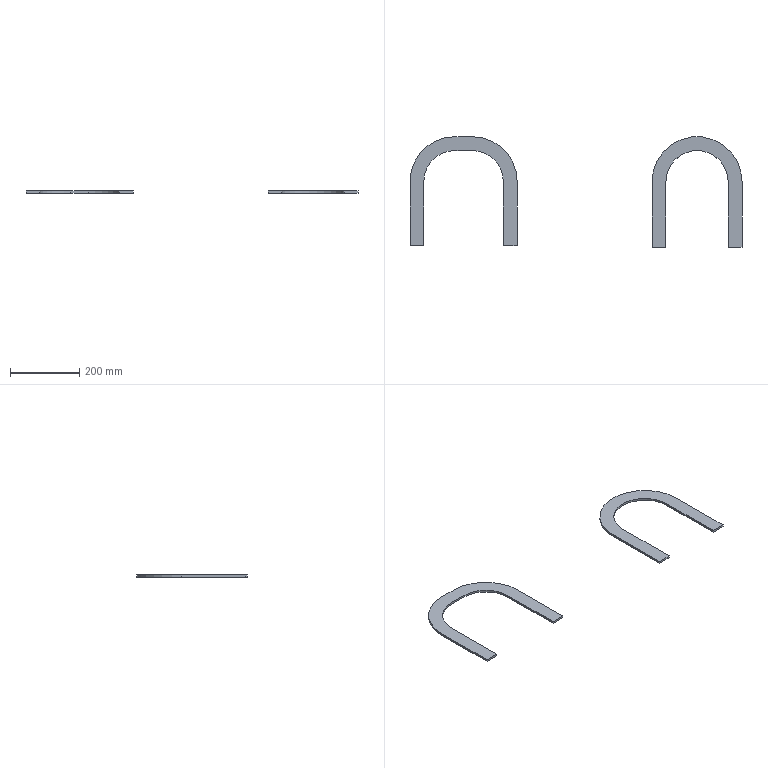Part | NX | features BREP 2 | 2 solids | 24 faces | box 960 x 320 x 6 mm | volume 357876 mm3 | plane 18 | cylinder 6 | commonest cylinder face diameters 180 x3 260 x3
STEP:
#1=CARTESIAN_POINT('',(130.,0.,0.));
#2=VERTEX_POINT('',#1);
#3=CARTESIAN_POINT('',(-130.,0.,0.));
#4=VERTEX_POINT('',#3);
#5=CARTESIAN_POINT('',(0.,0.,0.));
#6=DIRECTION('',(0.,0.,1.));
#7=DIRECTION('',(1.,0.,0.));
#8=AXIS2_PLACEMENT_3D('',#5,#6,#7);
#9=CIRCLE('',#8,130.);
#10=EDGE_CURVE('',#2,#4,#9,.T.);
#11=ORIENTED_EDGE('',*,*,#10,.T.);
#12=CARTESIAN_POINT('',(-130.,0.,6.));
#13=VERTEX_POINT('',#12);
#14=CARTESIAN_POINT('',(-130.,0.,6.));
#15=DIRECTION('',(0.,0.,-1.));
#16=VECTOR('',#15,1000.);
#17=LINE('',#14,#16);
#18=EDGE_CURVE('',#13,#4,#17,.T.);
#19=ORIENTED_EDGE('',*,*,#18,.F.);
#20=CARTESIAN_POINT('',(130.,0.,6.));
#21=VERTEX_POINT('',#20);
#22=CARTESIAN_POINT('',(0.,0.,6.));
#23=DIRECTION('',(0.,0.,1.));
#24=DIRECTION('',(1.,0.,0.));
#25=AXIS2_PLACEMENT_3D('',#22,#23,#24);
#26=CIRCLE('',#25,130.);
#27=EDGE_CURVE('',#21,#13,#26,.T.);
#28=ORIENTED_EDGE('',*,*,#27,.F.);
#29=CARTESIAN_POINT('',(130.,0.,6.));
#30=DIRECTION('',(0.,0.,-1.));
#31=VECTOR('',#30,1000.);
#32=LINE('',#29,#31);
#33=EDGE_CURVE('',#21,#2,#32,.T.);
#34=ORIENTED_EDGE('',*,*,#33,.T.);
#35=EDGE_LOOP('',(#11,#19,#28,#34));
#36=FACE_BOUND('',#35,.T.);
#37=CARTESIAN_POINT('',(0.,0.,6.));
#38=DIRECTION('',(0.,0.,-1.));
#39=DIRECTION('',(1.,0.,0.));
#40=AXIS2_PLACEMENT_3D('',#37,#38,#39);
#41=CYLINDRICAL_SURFACE('',#40,130.);
#42=ADVANCED_FACE('',(#36),#41,.T.);
#43=CARTESIAN_POINT('',(-130.,-190.,0.));
#44=VERTEX_POINT('',#43);
#45=CARTESIAN_POINT('',(-130.,-190.,0.));
#46=DIRECTION('',(0.,-1.,0.));
#47=VECTOR('',#46,1000.);
#48=LINE('',#45,#47);
#49=EDGE_CURVE('',#4,#44,#48,.T.);
#50=ORIENTED_EDGE('',*,*,#49,.T.);
#51=CARTESIAN_POINT('',(-130.,-190.,6.));
#52=VERTEX_POINT('',#51);
#53=CARTESIAN_POINT('',(-130.,-190.,6.));
#54=DIRECTION('',(0.,0.,-1.));
#55=VECTOR('',#54,1000.);
#56=LINE('',#53,#55);
#57=EDGE_CURVE('',#52,#44,#56,.T.);
#58=ORIENTED_EDGE('',*,*,#57,.F.);
#59=CARTESIAN_POINT('',(-130.,-190.,6.));
#60=DIRECTION('',(0.,-1.,0.));
#61=VECTOR('',#60,1000.);
#62=LINE('',#59,#61);
#63=EDGE_CURVE('',#13,#52,#62,.T.);
#64=ORIENTED_EDGE('',*,*,#63,.F.);
#65=ORIENTED_EDGE('',*,*,#18,.T.);
#66=EDGE_LOOP('',(#50,#58,#64,#65));
#67=FACE_BOUND('',#66,.T.);
#68=CARTESIAN_POINT('',(-130.,-190.,6.));
#69=DIRECTION('',(1.,0.,0.));
#70=DIRECTION('',(0.,-1.,0.));
#71=AXIS2_PLACEMENT_3D('',#68,#69,#70);
#72=PLANE('',#71);
#73=ADVANCED_FACE('',(#67),#72,.F.);
#74=CARTESIAN_POINT('',(-90.,-190.,0.));
#75=VERTEX_POINT('',#74);
#76=CARTESIAN_POINT('',(-90.,-190.,0.));
#77=DIRECTION('',(1.,0.,0.));
#78=VECTOR('',#77,1000.);
#79=LINE('',#76,#78);
#80=EDGE_CURVE('',#44,#75,#79,.T.);
#81=ORIENTED_EDGE('',*,*,#80,.T.);
#82=CARTESIAN_POINT('',(-90.,-190.,6.));
#83=VERTEX_POINT('',#82);
#84=CARTESIAN_POINT('',(-90.,-190.,6.));
#85=DIRECTION('',(0.,0.,-1.));
#86=VECTOR('',#85,1000.);
#87=LINE('',#84,#86);
#88=EDGE_CURVE('',#83,#75,#87,.T.);
#89=ORIENTED_EDGE('',*,*,#88,.F.);
#90=CARTESIAN_POINT('',(-90.,-190.,6.));
#91=DIRECTION('',(1.,0.,0.));
#92=VECTOR('',#91,1000.);
#93=LINE('',#90,#92);
#94=EDGE_CURVE('',#52,#83,#93,.T.);
#95=ORIENTED_EDGE('',*,*,#94,.F.);
#96=ORIENTED_EDGE('',*,*,#57,.T.);
#97=EDGE_LOOP('',(#81,#89,#95,#96));
#98=FACE_BOUND('',#97,.T.);
#99=CARTESIAN_POINT('',(-90.,-190.,6.));
#100=DIRECTION('',(0.,1.,0.));
#101=DIRECTION('',(0.,0.,-1.));
#102=AXIS2_PLACEMENT_3D('',#99,#100,#101);
#103=PLANE('',#102);
#104=ADVANCED_FACE('',(#98),#103,.F.);
#105=CARTESIAN_POINT('',(-90.,0.,0.));
#106=VERTEX_POINT('',#105);
#107=CARTESIAN_POINT('',(-90.,-190.,0.));
#108=DIRECTION('',(0.,1.,0.));
#109=VECTOR('',#108,1000.);
#110=LINE('',#107,#109);
#111=EDGE_CURVE('',#75,#106,#110,.T.);
#112=ORIENTED_EDGE('',*,*,#111,.T.);
#113=CARTESIAN_POINT('',(-90.,0.,6.));
#114=VERTEX_POINT('',#113);
#115=CARTESIAN_POINT('',(-90.,0.,6.));
#116=DIRECTION('',(0.,0.,-1.));
#117=VECTOR('',#116,1000.);
#118=LINE('',#115,#117);
#119=EDGE_CURVE('',#114,#106,#118,.T.);
#120=ORIENTED_EDGE('',*,*,#119,.F.);
#121=CARTESIAN_POINT('',(-90.,-190.,6.));
#122=DIRECTION('',(0.,1.,0.));
#123=VECTOR('',#122,1000.);
#124=LINE('',#121,#123);
#125=EDGE_CURVE('',#83,#114,#124,.T.);
#126=ORIENTED_EDGE('',*,*,#125,.F.);
#127=ORIENTED_EDGE('',*,*,#88,.T.);
#128=EDGE_LOOP('',(#112,#120,#126,#127));
#129=FACE_BOUND('',#128,.T.);
#130=CARTESIAN_POINT('',(-90.,-190.,6.));
#131=DIRECTION('',(-1.,0.,0.));
#132=DIRECTION('',(0.,0.,-1.));
#133=AXIS2_PLACEMENT_3D('',#130,#131,#132);
#134=PLANE('',#133);
#135=ADVANCED_FACE('',(#129),#134,.F.);
#136=CARTESIAN_POINT('',(90.,0.,0.));
#137=VERTEX_POINT('',#136);
#138=CARTESIAN_POINT('',(0.,0.,0.));
#139=DIRECTION('',(0.,0.,-1.));
#140=DIRECTION('',(1.,0.,0.));
#141=AXIS2_PLACEMENT_3D('',#138,#139,#140);
#142=CIRCLE('',#141,90.);
#143=EDGE_CURVE('',#106,#137,#142,.T.);
#144=ORIENTED_EDGE('',*,*,#143,.T.);
#145=CARTESIAN_POINT('',(90.,0.,6.));
#146=VERTEX_POINT('',#145);
#147=CARTESIAN_POINT('',(90.,0.,6.));
#148=DIRECTION('',(0.,0.,-1.));
#149=VECTOR('',#148,1000.);
#150=LINE('',#147,#149);
#151=EDGE_CURVE('',#146,#137,#150,.T.);
#152=ORIENTED_EDGE('',*,*,#151,.F.);
#153=CARTESIAN_POINT('',(0.,0.,6.));
#154=DIRECTION('',(0.,0.,-1.));
#155=DIRECTION('',(1.,0.,0.));
#156=AXIS2_PLACEMENT_3D('',#153,#154,#155);
#157=CIRCLE('',#156,90.);
#158=EDGE_CURVE('',#114,#146,#157,.T.);
#159=ORIENTED_EDGE('',*,*,#158,.F.);
#160=ORIENTED_EDGE('',*,*,#119,.T.);
#161=EDGE_LOOP('',(#144,#152,#159,#160));
#162=FACE_BOUND('',#161,.T.);
#163=CARTESIAN_POINT('',(0.,0.,6.));
#164=DIRECTION('',(0.,0.,-1.));
#165=DIRECTION('',(1.,0.,0.));
#166=AXIS2_PLACEMENT_3D('',#163,#164,#165);
#167=CYLINDRICAL_SURFACE('',#166,90.);
#168=ADVANCED_FACE('',(#162),#167,.F.);
#169=CARTESIAN_POINT('',(90.,-190.,0.));
#170=VERTEX_POINT('',#169);
#171=CARTESIAN_POINT('',(90.,0.,0.));
#172=DIRECTION('',(0.,-1.,0.));
#173=VECTOR('',#172,1000.);
#174=LINE('',#171,#173);
#175=EDGE_CURVE('',#137,#170,#174,.T.);
#176=ORIENTED_EDGE('',*,*,#175,.T.);
#177=CARTESIAN_POINT('',(90.,-190.,6.));
#178=VERTEX_POINT('',#177);
#179=CARTESIAN_POINT('',(90.,-190.,6.));
#180=DIRECTION('',(0.,0.,-1.));
#181=VECTOR('',#180,1000.);
#182=LINE('',#179,#181);
#183=EDGE_CURVE('',#178,#170,#182,.T.);
#184=ORIENTED_EDGE('',*,*,#183,.F.);
#185=CARTESIAN_POINT('',(90.,0.,6.));
#186=DIRECTION('',(0.,-1.,0.));
#187=VECTOR('',#186,1000.);
#188=LINE('',#185,#187);
#189=EDGE_CURVE('',#146,#178,#188,.T.);
#190=ORIENTED_EDGE('',*,*,#189,.F.);
#191=ORIENTED_EDGE('',*,*,#151,.T.);
#192=EDGE_LOOP('',(#176,#184,#190,#191));
#193=FACE_BOUND('',#192,.T.);
#194=CARTESIAN_POINT('',(90.,0.,6.));
#195=DIRECTION('',(1.,0.,0.));
#196=DIRECTION('',(0.,0.,1.));
#197=AXIS2_PLACEMENT_3D('',#194,#195,#196);
#198=PLANE('',#197);
#199=ADVANCED_FACE('',(#193),#198,.F.);
#200=CARTESIAN_POINT('',(130.,-190.,0.));
#201=VERTEX_POINT('',#200);
#202=CARTESIAN_POINT('',(90.,-190.,0.));
#203=DIRECTION('',(1.,0.,0.));
#204=VECTOR('',#203,1000.);
#205=LINE('',#202,#204);
#206=EDGE_CURVE('',#170,#201,#205,.T.);
#207=ORIENTED_EDGE('',*,*,#206,.T.);
#208=CARTESIAN_POINT('',(130.,-190.,6.));
#209=VERTEX_POINT('',#208);
#210=CARTESIAN_POINT('',(130.,-190.,6.));
#211=DIRECTION('',(0.,0.,-1.));
#212=VECTOR('',#211,1000.);
#213=LINE('',#210,#212);
#214=EDGE_CURVE('',#209,#201,#213,.T.);
#215=ORIENTED_EDGE('',*,*,#214,.F.);
#216=CARTESIAN_POINT('',(90.,-190.,6.));
#217=DIRECTION('',(1.,0.,0.));
#218=VECTOR('',#217,1000.);
#219=LINE('',#216,#218);
#220=EDGE_CURVE('',#178,#209,#219,.T.);
#221=ORIENTED_EDGE('',*,*,#220,.F.);
#222=ORIENTED_EDGE('',*,*,#183,.T.);
#223=EDGE_LOOP('',(#207,#215,#221,#222));
#224=FACE_BOUND('',#223,.T.);
#225=CARTESIAN_POINT('',(90.,-190.,6.));
#226=DIRECTION('',(0.,1.,0.));
#227=DIRECTION('',(0.,0.,-1.));
#228=AXIS2_PLACEMENT_3D('',#225,#226,#227);
#229=PLANE('',#228);
#230=ADVANCED_FACE('',(#224),#229,.F.);
#231=CARTESIAN_POINT('',(130.,0.,0.));
#232=DIRECTION('',(0.,1.,0.));
#233=VECTOR('',#232,1000.);
#234=LINE('',#231,#233);
#235=EDGE_CURVE('',#201,#2,#234,.T.);
#236=ORIENTED_EDGE('',*,*,#235,.T.);
#237=ORIENTED_EDGE('',*,*,#33,.F.);
#238=CARTESIAN_POINT('',(130.,0.,6.));
#239=DIRECTION('',(0.,1.,0.));
#240=VECTOR('',#239,1000.);
#241=LINE('',#238,#240);
#242=EDGE_CURVE('',#209,#21,#241,.T.);
#243=ORIENTED_EDGE('',*,*,#242,.F.);
#244=ORIENTED_EDGE('',*,*,#214,.T.);
#245=EDGE_LOOP('',(#236,#237,#243,#244));
#246=FACE_BOUND('',#245,.T.);
#247=CARTESIAN_POINT('',(130.,0.,6.));
#248=DIRECTION('',(-1.,0.,0.));
#249=DIRECTION('',(0.,0.,-1.));
#250=AXIS2_PLACEMENT_3D('',#247,#248,#249);
#251=PLANE('',#250);
#252=ADVANCED_FACE('',(#246),#251,.F.);
#253=ORIENTED_EDGE('',*,*,#27,.T.);
#254=ORIENTED_EDGE('',*,*,#63,.T.);
#255=ORIENTED_EDGE('',*,*,#94,.T.);
#256=ORIENTED_EDGE('',*,*,#125,.T.);
#257=ORIENTED_EDGE('',*,*,#158,.T.);
#258=ORIENTED_EDGE('',*,*,#189,.T.);
#259=ORIENTED_EDGE('',*,*,#220,.T.);
#260=ORIENTED_EDGE('',*,*,#242,.T.);
#261=EDGE_LOOP('',(#253,#254,#255,#256,#257,#258,#259,#260));
#262=FACE_BOUND('',#261,.T.);
#263=CARTESIAN_POINT('',(0.,0.,6.));
#264=DIRECTION('',(0.,0.,1.));
#265=DIRECTION('',(-1.,0.,0.));
#266=AXIS2_PLACEMENT_3D('',#263,#264,#265);
#267=PLANE('',#266);
#268=ADVANCED_FACE('',(#262),#267,.T.);
#269=ORIENTED_EDGE('',*,*,#10,.F.);
#270=ORIENTED_EDGE('',*,*,#235,.F.);
#271=ORIENTED_EDGE('',*,*,#206,.F.);
#272=ORIENTED_EDGE('',*,*,#175,.F.);
#273=ORIENTED_EDGE('',*,*,#143,.F.);
#274=ORIENTED_EDGE('',*,*,#111,.F.);
#275=ORIENTED_EDGE('',*,*,#80,.F.);
#276=ORIENTED_EDGE('',*,*,#49,.F.);
#277=EDGE_LOOP('',(#269,#270,#271,#272,#273,#274,#275,#276));
#278=FACE_BOUND('',#277,.T.);
#279=CARTESIAN_POINT('',(0.,0.,0.));
#280=DIRECTION('',(0.,0.,1.));
#281=DIRECTION('',(-1.,0.,0.));
#282=AXIS2_PLACEMENT_3D('',#279,#280,#281);
#283=PLANE('',#282);
#284=ADVANCED_FACE('',(#278),#283,.F.);
#285=CLOSED_SHELL('',(#42,#73,#104,#135,#168,#199,#230,#252,#268,#284));
#286=MANIFOLD_SOLID_BREP('',#285);
#287=CARTESIAN_POINT('',(-700.,130.,0.));
#288=VERTEX_POINT('',#287);
#289=CARTESIAN_POINT('',(-830.,0.,0.));
#290=VERTEX_POINT('',#289);
#291=CARTESIAN_POINT('',(-700.,0.,0.));
#292=DIRECTION('',(0.,0.,1.));
#293=DIRECTION('',(1.,0.,0.));
#294=AXIS2_PLACEMENT_3D('',#291,#292,#293);
#295=CIRCLE('',#294,130.);
#296=EDGE_CURVE('',#288,#290,#295,.T.);
#297=ORIENTED_EDGE('',*,*,#296,.T.);
#298=CARTESIAN_POINT('',(-830.,0.,6.));
#299=VERTEX_POINT('',#298);
#300=CARTESIAN_POINT('',(-830.,0.,6.));
#301=DIRECTION('',(0.,0.,-1.));
#302=VECTOR('',#301,1000.);
#303=LINE('',#300,#302);
#304=EDGE_CURVE('',#299,#290,#303,.T.);
#305=ORIENTED_EDGE('',*,*,#304,.F.);
#306=CARTESIAN_POINT('',(-700.,130.,6.));
#307=VERTEX_POINT('',#306);
#308=CARTESIAN_POINT('',(-700.,0.,6.));
#309=DIRECTION('',(0.,0.,1.));
#310=DIRECTION('',(1.,0.,0.));
#311=AXIS2_PLACEMENT_3D('',#308,#309,#310);
#312=CIRCLE('',#311,130.);
#313=EDGE_CURVE('',#307,#299,#312,.T.);
#314=ORIENTED_EDGE('',*,*,#313,.F.);
#315=CARTESIAN_POINT('',(-700.,130.,6.));
#316=DIRECTION('',(0.,0.,-1.));
#317=VECTOR('',#316,1000.);
#318=LINE('',#315,#317);
#319=EDGE_CURVE('',#307,#288,#318,.T.);
#320=ORIENTED_EDGE('',*,*,#319,.T.);
#321=EDGE_LOOP('',(#297,#305,#314,#320));
#322=FACE_BOUND('',#321,.T.);
#323=CARTESIAN_POINT('',(-700.,0.,6.));
#324=DIRECTION('',(0.,0.,-1.));
#325=DIRECTION('',(1.,0.,0.));
#326=AXIS2_PLACEMENT_3D('',#323,#324,#325);
#327=CYLINDRICAL_SURFACE('',#326,130.);
#328=ADVANCED_FACE('',(#322),#327,.T.);
#329=CARTESIAN_POINT('',(-830.,-185.,0.));
#330=VERTEX_POINT('',#329);
#331=CARTESIAN_POINT('',(-830.,-185.,0.));
#332=DIRECTION('',(0.,-1.,0.));
#333=VECTOR('',#332,1000.);
#334=LINE('',#331,#333);
#335=EDGE_CURVE('',#290,#330,#334,.T.);
#336=ORIENTED_EDGE('',*,*,#335,.T.);
#337=CARTESIAN_POINT('',(-830.,-185.,6.));
#338=VERTEX_POINT('',#337);
#339=CARTESIAN_POINT('',(-830.,-185.,6.));
#340=DIRECTION('',(0.,0.,-1.));
#341=VECTOR('',#340,1000.);
#342=LINE('',#339,#341);
#343=EDGE_CURVE('',#338,#330,#342,.T.);
#344=ORIENTED_EDGE('',*,*,#343,.F.);
#345=CARTESIAN_POINT('',(-830.,-185.,6.));
#346=DIRECTION('',(0.,-1.,0.));
#347=VECTOR('',#346,1000.);
#348=LINE('',#345,#347);
#349=EDGE_CURVE('',#299,#338,#348,.T.);
#350=ORIENTED_EDGE('',*,*,#349,.F.);
#351=ORIENTED_EDGE('',*,*,#304,.T.);
#352=EDGE_LOOP('',(#336,#344,#350,#351));
#353=FACE_BOUND('',#352,.T.);
#354=CARTESIAN_POINT('',(-830.,-185.,6.));
#355=DIRECTION('',(1.,0.,0.));
#356=DIRECTION('',(0.,0.,1.));
#357=AXIS2_PLACEMENT_3D('',#354,#355,#356);
#358=PLANE('',#357);
#359=ADVANCED_FACE('',(#353),#358,.F.);
#360=CARTESIAN_POINT('',(-790.,-185.,0.));
#361=VERTEX_POINT('',#360);
#362=CARTESIAN_POINT('',(-830.,-185.,0.));
#363=DIRECTION('',(1.,0.,0.));
#364=VECTOR('',#363,1000.);
#365=LINE('',#362,#364);
#366=EDGE_CURVE('',#330,#361,#365,.T.);
#367=ORIENTED_EDGE('',*,*,#366,.T.);
#368=CARTESIAN_POINT('',(-790.,-185.,6.));
#369=VERTEX_POINT('',#368);
#370=CARTESIAN_POINT('',(-790.,-185.,6.));
#371=DIRECTION('',(0.,0.,-1.));
#372=VECTOR('',#371,1000.);
#373=LINE('',#370,#372);
#374=EDGE_CURVE('',#369,#361,#373,.T.);
#375=ORIENTED_EDGE('',*,*,#374,.F.);
#376=CARTESIAN_POINT('',(-830.,-185.,6.));
#377=DIRECTION('',(1.,0.,0.));
#378=VECTOR('',#377,1000.);
#379=LINE('',#376,#378);
#380=EDGE_CURVE('',#338,#369,#379,.T.);
#381=ORIENTED_EDGE('',*,*,#380,.F.);
#382=ORIENTED_EDGE('',*,*,#343,.T.);
#383=EDGE_LOOP('',(#367,#375,#381,#382));
#384=FACE_BOUND('',#383,.T.);
#385=CARTESIAN_POINT('',(-830.,-185.,6.));
#386=DIRECTION('',(0.,1.,0.));
#387=DIRECTION('',(0.,0.,-1.));
#388=AXIS2_PLACEMENT_3D('',#385,#386,#387);
#389=PLANE('',#388);
#390=ADVANCED_FACE('',(#384),#389,.F.);
#391=CARTESIAN_POINT('',(-790.,0.,0.));
#392=VERTEX_POINT('',#391);
#393=CARTESIAN_POINT('',(-790.,-185.,0.));
#394=DIRECTION('',(0.,1.,0.));
#395=VECTOR('',#394,1000.);
#396=LINE('',#393,#395);
#397=EDGE_CURVE('',#361,#392,#396,.T.);
#398=ORIENTED_EDGE('',*,*,#397,.T.);
#399=CARTESIAN_POINT('',(-790.,0.,6.));
#400=VERTEX_POINT('',#399);
#401=CARTESIAN_POINT('',(-790.,0.,6.));
#402=DIRECTION('',(0.,0.,-1.));
#403=VECTOR('',#402,1000.);
#404=LINE('',#401,#403);
#405=EDGE_CURVE('',#400,#392,#404,.T.);
#406=ORIENTED_EDGE('',*,*,#405,.F.);
#407=CARTESIAN_POINT('',(-790.,-185.,6.));
#408=DIRECTION('',(0.,1.,0.));
#409=VECTOR('',#408,1000.);
#410=LINE('',#407,#409);
#411=EDGE_CURVE('',#369,#400,#410,.T.);
#412=ORIENTED_EDGE('',*,*,#411,.F.);
#413=ORIENTED_EDGE('',*,*,#374,.T.);
#414=EDGE_LOOP('',(#398,#406,#412,#413));
#415=FACE_BOUND('',#414,.T.);
#416=CARTESIAN_POINT('',(-790.,-185.,6.));
#417=DIRECTION('',(-1.,0.,0.));
#418=DIRECTION('',(0.,0.,-1.));
#419=AXIS2_PLACEMENT_3D('',#416,#417,#418);
#420=PLANE('',#419);
#421=ADVANCED_FACE('',(#415),#420,.F.);
#422=CARTESIAN_POINT('',(-700.,90.,0.));
#423=VERTEX_POINT('',#422);
#424=CARTESIAN_POINT('',(-700.,0.,0.));
#425=DIRECTION('',(0.,0.,-1.));
#426=DIRECTION('',(1.,0.,0.));
#427=AXIS2_PLACEMENT_3D('',#424,#425,#426);
#428=CIRCLE('',#427,90.);
#429=EDGE_CURVE('',#392,#423,#428,.T.);
#430=ORIENTED_EDGE('',*,*,#429,.T.);
#431=CARTESIAN_POINT('',(-700.,90.,6.));
#432=VERTEX_POINT('',#431);
#433=CARTESIAN_POINT('',(-700.,90.,6.));
#434=DIRECTION('',(0.,0.,-1.));
#435=VECTOR('',#434,1000.);
#436=LINE('',#433,#435);
#437=EDGE_CURVE('',#432,#423,#436,.T.);
#438=ORIENTED_EDGE('',*,*,#437,.F.);
#439=CARTESIAN_POINT('',(-700.,0.,6.));
#440=DIRECTION('',(0.,0.,-1.));
#441=DIRECTION('',(1.,0.,0.));
#442=AXIS2_PLACEMENT_3D('',#439,#440,#441);
#443=CIRCLE('',#442,90.);
#444=EDGE_CURVE('',#400,#432,#443,.T.);
#445=ORIENTED_EDGE('',*,*,#444,.F.);
#446=ORIENTED_EDGE('',*,*,#405,.T.);
#447=EDGE_LOOP('',(#430,#438,#445,#446));
#448=FACE_BOUND('',#447,.T.);
#449=CARTESIAN_POINT('',(-700.,0.,6.));
#450=DIRECTION('',(0.,0.,-1.));
#451=DIRECTION('',(1.,0.,0.));
#452=AXIS2_PLACEMENT_3D('',#449,#450,#451);
#453=CYLINDRICAL_SURFACE('',#452,90.);
#454=ADVANCED_FACE('',(#448),#453,.F.);
#455=CARTESIAN_POINT('',(-650.,90.,0.));
#456=VERTEX_POINT('',#455);
#457=CARTESIAN_POINT('',(-700.,90.,0.));
#458=DIRECTION('',(1.,0.,0.));
#459=VECTOR('',#458,1000.);
#460=LINE('',#457,#459);
#461=EDGE_CURVE('',#423,#456,#460,.T.);
#462=ORIENTED_EDGE('',*,*,#461,.T.);
#463=CARTESIAN_POINT('',(-650.,90.,6.));
#464=VERTEX_POINT('',#463);
#465=CARTESIAN_POINT('',(-650.,90.,6.));
#466=DIRECTION('',(0.,0.,-1.));
#467=VECTOR('',#466,1000.);
#468=LINE('',#465,#467);
#469=EDGE_CURVE('',#464,#456,#468,.T.);
#470=ORIENTED_EDGE('',*,*,#469,.F.);
#471=CARTESIAN_POINT('',(-700.,90.,6.));
#472=DIRECTION('',(1.,0.,0.));
#473=VECTOR('',#472,1000.);
#474=LINE('',#471,#473);
#475=EDGE_CURVE('',#432,#464,#474,.T.);
#476=ORIENTED_EDGE('',*,*,#475,.F.);
#477=ORIENTED_EDGE('',*,*,#437,.T.);
#478=EDGE_LOOP('',(#462,#470,#476,#477));
#479=FACE_BOUND('',#478,.T.);
#480=CARTESIAN_POINT('',(-700.,90.,6.));
#481=DIRECTION('',(0.,1.,0.));
#482=DIRECTION('',(1.,0.,0.));
#483=AXIS2_PLACEMENT_3D('',#480,#481,#482);
#484=PLANE('',#483);
#485=ADVANCED_FACE('',(#479),#484,.F.);
#486=CARTESIAN_POINT('',(-560.,0.,0.));
#487=VERTEX_POINT('',#486);
#488=CARTESIAN_POINT('',(-650.,0.,0.));
#489=DIRECTION('',(0.,0.,-1.));
#490=DIRECTION('',(1.,0.,0.));
#491=AXIS2_PLACEMENT_3D('',#488,#489,#490);
#492=CIRCLE('',#491,90.);
#493=EDGE_CURVE('',#456,#487,#492,.T.);
#494=ORIENTED_EDGE('',*,*,#493,.T.);
#495=CARTESIAN_POINT('',(-560.,0.,6.));
#496=VERTEX_POINT('',#495);
#497=CARTESIAN_POINT('',(-560.,0.,6.));
#498=DIRECTION('',(0.,0.,-1.));
#499=VECTOR('',#498,1000.);
#500=LINE('',#497,#499);
#501=EDGE_CURVE('',#496,#487,#500,.T.);
#502=ORIENTED_EDGE('',*,*,#501,.F.);
#503=CARTESIAN_POINT('',(-650.,0.,6.));
#504=DIRECTION('',(0.,0.,-1.));
#505=DIRECTION('',(1.,0.,0.));
#506=AXIS2_PLACEMENT_3D('',#503,#504,#505);
#507=CIRCLE('',#506,90.);
#508=EDGE_CURVE('',#464,#496,#507,.T.);
#509=ORIENTED_EDGE('',*,*,#508,.F.);
#510=ORIENTED_EDGE('',*,*,#469,.T.);
#511=EDGE_LOOP('',(#494,#502,#509,#510));
#512=FACE_BOUND('',#511,.T.);
#513=CARTESIAN_POINT('',(-650.,0.,6.));
#514=DIRECTION('',(0.,0.,-1.));
#515=DIRECTION('',(1.,0.,0.));
#516=AXIS2_PLACEMENT_3D('',#513,#514,#515);
#517=CYLINDRICAL_SURFACE('',#516,90.);
#518=ADVANCED_FACE('',(#512),#517,.F.);
#519=CARTESIAN_POINT('',(-560.,-185.,0.));
#520=VERTEX_POINT('',#519);
#521=CARTESIAN_POINT('',(-560.,0.,0.));
#522=DIRECTION('',(0.,-1.,0.));
#523=VECTOR('',#522,1000.);
#524=LINE('',#521,#523);
#525=EDGE_CURVE('',#487,#520,#524,.T.);
#526=ORIENTED_EDGE('',*,*,#525,.T.);
#527=CARTESIAN_POINT('',(-560.,-185.,6.));
#528=VERTEX_POINT('',#527);
#529=CARTESIAN_POINT('',(-560.,-185.,6.));
#530=DIRECTION('',(0.,0.,-1.));
#531=VECTOR('',#530,1000.);
#532=LINE('',#529,#531);
#533=EDGE_CURVE('',#528,#520,#532,.T.);
#534=ORIENTED_EDGE('',*,*,#533,.F.);
#535=CARTESIAN_POINT('',(-560.,0.,6.));
#536=DIRECTION('',(0.,-1.,0.));
#537=VECTOR('',#536,1000.);
#538=LINE('',#535,#537);
#539=EDGE_CURVE('',#496,#528,#538,.T.);
#540=ORIENTED_EDGE('',*,*,#539,.F.);
#541=ORIENTED_EDGE('',*,*,#501,.T.);
#542=EDGE_LOOP('',(#526,#534,#540,#541));
#543=FACE_BOUND('',#542,.T.);
#544=CARTESIAN_POINT('',(-560.,0.,6.));
#545=DIRECTION('',(1.,0.,0.));
#546=DIRECTION('',(0.,0.,1.));
#547=AXIS2_PLACEMENT_3D('',#544,#545,#546);
#548=PLANE('',#547);
#549=ADVANCED_FACE('',(#543),#548,.F.);
#550=CARTESIAN_POINT('',(-520.,-185.,0.));
#551=VERTEX_POINT('',#550);
#552=CARTESIAN_POINT('',(-560.,-185.,0.));
#553=DIRECTION('',(1.,0.,0.));
#554=VECTOR('',#553,1000.);
#555=LINE('',#552,#554);
#556=EDGE_CURVE('',#520,#551,#555,.T.);
#557=ORIENTED_EDGE('',*,*,#556,.T.);
#558=CARTESIAN_POINT('',(-520.,-185.,6.));
#559=VERTEX_POINT('',#558);
#560=CARTESIAN_POINT('',(-520.,-185.,6.));
#561=DIRECTION('',(0.,0.,-1.));
#562=VECTOR('',#561,1000.);
#563=LINE('',#560,#562);
#564=EDGE_CURVE('',#559,#551,#563,.T.);
#565=ORIENTED_EDGE('',*,*,#564,.F.);
#566=CARTESIAN_POINT('',(-560.,-185.,6.));
#567=DIRECTION('',(1.,0.,0.));
#568=VECTOR('',#567,1000.);
#569=LINE('',#566,#568);
#570=EDGE_CURVE('',#528,#559,#569,.T.);
#571=ORIENTED_EDGE('',*,*,#570,.F.);
#572=ORIENTED_EDGE('',*,*,#533,.T.);
#573=EDGE_LOOP('',(#557,#565,#571,#572));
#574=FACE_BOUND('',#573,.T.);
#575=CARTESIAN_POINT('',(-560.,-185.,6.));
#576=DIRECTION('',(0.,1.,0.));
#577=DIRECTION('',(0.,0.,-1.));
#578=AXIS2_PLACEMENT_3D('',#575,#576,#577);
#579=PLANE('',#578);
#580=ADVANCED_FACE('',(#574),#579,.F.);
#581=CARTESIAN_POINT('',(-520.,0.,0.));
#582=VERTEX_POINT('',#581);
#583=CARTESIAN_POINT('',(-520.,0.,0.));
#584=DIRECTION('',(0.,1.,0.));
#585=VECTOR('',#584,1000.);
#586=LINE('',#583,#585);
#587=EDGE_CURVE('',#551,#582,#586,.T.);
#588=ORIENTED_EDGE('',*,*,#587,.T.);
#589=CARTESIAN_POINT('',(-520.,0.,6.));
#590=VERTEX_POINT('',#589);
#591=CARTESIAN_POINT('',(-520.,0.,6.));
#592=DIRECTION('',(0.,0.,-1.));
#593=VECTOR('',#592,1000.);
#594=LINE('',#591,#593);
#595=EDGE_CURVE('',#590,#582,#594,.T.);
#596=ORIENTED_EDGE('',*,*,#595,.F.);
#597=CARTESIAN_POINT('',(-520.,0.,6.));
#598=DIRECTION('',(0.,1.,0.));
#599=VECTOR('',#598,1000.);
#600=LINE('',#597,#599);
#601=EDGE_CURVE('',#559,#590,#600,.T.);
#602=ORIENTED_EDGE('',*,*,#601,.F.);
#603=ORIENTED_EDGE('',*,*,#564,.T.);
#604=EDGE_LOOP('',(#588,#596,#602,#603));
#605=FACE_BOUND('',#604,.T.);
#606=CARTESIAN_POINT('',(-520.,0.,6.));
#607=DIRECTION('',(-1.,0.,0.));
#608=DIRECTION('',(0.,0.,-1.));
#609=AXIS2_PLACEMENT_3D('',#606,#607,#608);
#610=PLANE('',#609);
#611=ADVANCED_FACE('',(#605),#610,.F.);
#612=CARTESIAN_POINT('',(-650.,130.,0.));
#613=VERTEX_POINT('',#612);
#614=CARTESIAN_POINT('',(-650.,0.,0.));
#615=DIRECTION('',(0.,0.,1.));
#616=DIRECTION('',(1.,0.,0.));
#617=AXIS2_PLACEMENT_3D('',#614,#615,#616);
#618=CIRCLE('',#617,130.);
#619=EDGE_CURVE('',#582,#613,#618,.T.);
#620=ORIENTED_EDGE('',*,*,#619,.T.);
#621=CARTESIAN_POINT('',(-650.,130.,6.));
#622=VERTEX_POINT('',#621);
#623=CARTESIAN_POINT('',(-650.,130.,6.));
#624=DIRECTION('',(0.,0.,-1.));
#625=VECTOR('',#624,1000.);
#626=LINE('',#623,#625);
#627=EDGE_CURVE('',#622,#613,#626,.T.);
#628=ORIENTED_EDGE('',*,*,#627,.F.);
#629=CARTESIAN_POINT('',(-650.,0.,6.));
#630=DIRECTION('',(0.,0.,1.));
#631=DIRECTION('',(1.,0.,0.));
#632=AXIS2_PLACEMENT_3D('',#629,#630,#631);
#633=CIRCLE('',#632,130.);
#634=EDGE_CURVE('',#590,#622,#633,.T.);
#635=ORIENTED_EDGE('',*,*,#634,.F.);
#636=ORIENTED_EDGE('',*,*,#595,.T.);
#637=EDGE_LOOP('',(#620,#628,#635,#636));
#638=FACE_BOUND('',#637,.T.);
#639=CARTESIAN_POINT('',(-650.,0.,6.));
#640=DIRECTION('',(0.,0.,-1.));
#641=DIRECTION('',(1.,0.,0.));
#642=AXIS2_PLACEMENT_3D('',#639,#640,#641);
#643=CYLINDRICAL_SURFACE('',#642,130.);
#644=ADVANCED_FACE('',(#638),#643,.T.);
#645=CARTESIAN_POINT('',(-700.,130.,0.));
#646=DIRECTION('',(-1.,0.,0.));
#647=VECTOR('',#646,1000.);
#648=LINE('',#645,#647);
#649=EDGE_CURVE('',#613,#288,#648,.T.);
#650=ORIENTED_EDGE('',*,*,#649,.T.);
#651=ORIENTED_EDGE('',*,*,#319,.F.);
#652=CARTESIAN_POINT('',(-700.,130.,6.));
#653=DIRECTION('',(-1.,0.,0.));
#654=VECTOR('',#653,1000.);
#655=LINE('',#652,#654);
#656=EDGE_CURVE('',#622,#307,#655,.T.);
#657=ORIENTED_EDGE('',*,*,#656,.F.);
#658=ORIENTED_EDGE('',*,*,#627,.T.);
#659=EDGE_LOOP('',(#650,#651,#657,#658));
#660=FACE_BOUND('',#659,.T.);
#661=CARTESIAN_POINT('',(-700.,130.,6.));
#662=DIRECTION('',(0.,-1.,0.));
#663=DIRECTION('',(0.,0.,1.));
#664=AXIS2_PLACEMENT_3D('',#661,#662,#663);
#665=PLANE('',#664);
#666=ADVANCED_FACE('',(#660),#665,.F.);
#667=ORIENTED_EDGE('',*,*,#313,.T.);
#668=ORIENTED_EDGE('',*,*,#349,.T.);
#669=ORIENTED_EDGE('',*,*,#380,.T.);
#670=ORIENTED_EDGE('',*,*,#411,.T.);
#671=ORIENTED_EDGE('',*,*,#444,.T.);
#672=ORIENTED_EDGE('',*,*,#475,.T.);
#673=ORIENTED_EDGE('',*,*,#508,.T.);
#674=ORIENTED_EDGE('',*,*,#539,.T.);
#675=ORIENTED_EDGE('',*,*,#570,.T.);
#676=ORIENTED_EDGE('',*,*,#601,.T.);
#677=ORIENTED_EDGE('',*,*,#634,.T.);
#678=ORIENTED_EDGE('',*,*,#656,.T.);
#679=EDGE_LOOP('',(#667,#668,#669,#670,#671,#672,#673,#674,#675,#676,#677,#678));
#680=FACE_BOUND('',#679,.T.);
#681=CARTESIAN_POINT('',(-700.,0.,6.));
#682=DIRECTION('',(0.,0.,1.));
#683=DIRECTION('',(-1.,0.,0.));
#684=AXIS2_PLACEMENT_3D('',#681,#682,#683);
#685=PLANE('',#684);
#686=ADVANCED_FACE('',(#680),#685,.T.);
#687=ORIENTED_EDGE('',*,*,#296,.F.);
#688=ORIENTED_EDGE('',*,*,#649,.F.);
#689=ORIENTED_EDGE('',*,*,#619,.F.);
#690=ORIENTED_EDGE('',*,*,#587,.F.);
#691=ORIENTED_EDGE('',*,*,#556,.F.);
#692=ORIENTED_EDGE('',*,*,#525,.F.);
#693=ORIENTED_EDGE('',*,*,#493,.F.);
#694=ORIENTED_EDGE('',*,*,#461,.F.);
#695=ORIENTED_EDGE('',*,*,#429,.F.);
#696=ORIENTED_EDGE('',*,*,#397,.F.);
#697=ORIENTED_EDGE('',*,*,#366,.F.);
#698=ORIENTED_EDGE('',*,*,#335,.F.);
#699=EDGE_LOOP('',(#687,#688,#689,#690,#691,#692,#693,#694,#695,#696,#697,#698));
#700=FACE_BOUND('',#699,.T.);
#701=CARTESIAN_POINT('',(-700.,0.,0.));
#702=DIRECTION('',(0.,0.,1.));
#703=DIRECTION('',(-1.,0.,0.));
#704=AXIS2_PLACEMENT_3D('',#701,#702,#703);
#705=PLANE('',#704);
#706=ADVANCED_FACE('',(#700),#705,.F.);
#707=CLOSED_SHELL('',(#328,#359,#390,#421,#454,#485,#518,#549,#580,#611,#644,#666,#686,#706));
#708=MANIFOLD_SOLID_BREP('',#707);
#709=(LENGTH_UNIT()NAMED_UNIT(*)SI_UNIT(.MILLI.,.METRE.));
#710=UNCERTAINTY_MEASURE_WITH_UNIT(LENGTH_MEASURE(0.00001),#709,'','');
#711=(NAMED_UNIT(*)PLANE_ANGLE_UNIT()SI_UNIT($,.RADIAN.));
#712=(NAMED_UNIT(*)SI_UNIT($,.STERADIAN.)SOLID_ANGLE_UNIT());
#713=(GEOMETRIC_REPRESENTATION_CONTEXT(3)GLOBAL_UNCERTAINTY_ASSIGNED_CONTEXT((#710))GLOBAL_UNIT_ASSIGNED_CONTEXT((#709,#711,#712))REPRESENTATION_CONTEXT('',''));
#714=ADVANCED_BREP_SHAPE_REPRESENTATION('',(#286,#708),#713);